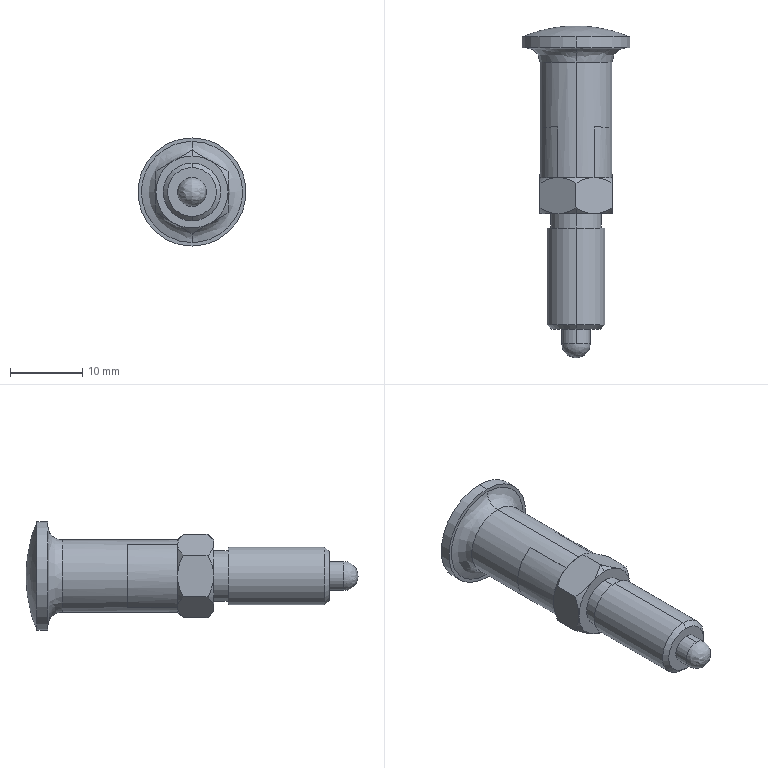Part | SolidWorks | features BaseBody 1 | 1 solid | 49 faces | box 15 x 46 x 15 mm | volume 3087 mm3 | plane 18 | cone 15 | cylinder 12 | spline 4 | commonest cylinder face diameters 4 x2 7 x2 8 x2 9.98 x2 10 x2 15 x2